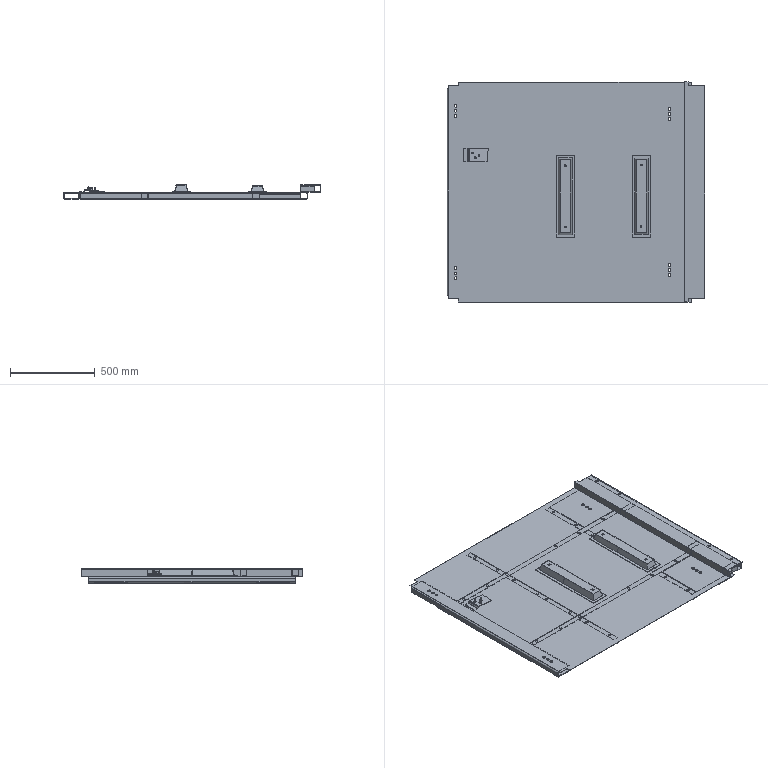Part | NX | features BREP 16 | 31 solids | 1066 faces | box 1524 x 1300 x 84.135 mm | volume 9485940 mm3 | cylinder 488 | plane 487 | cone 33 | torus 27 | sphere 27 | spline 4 | commonest cylinder face diameters 15 x144 6 x116 10 x64 17 x56 8 x34 9 x16